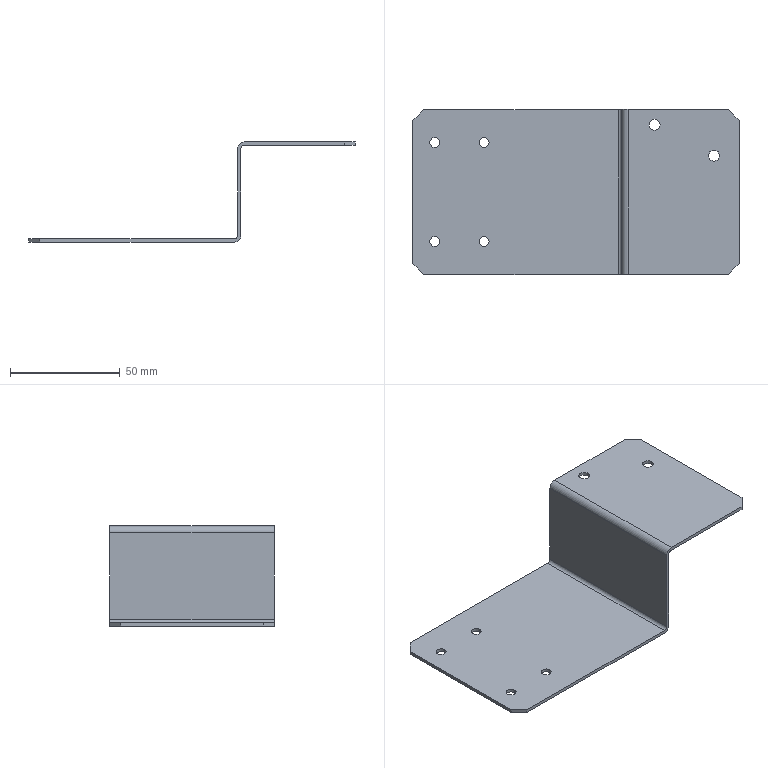Part | STEP file | 866-BDO024-96-03A_default | 1 solid | 30 faces | box 148.5 x 75 x 45.5 mm | volume 21210 mm3 | cylinder 16 | plane 14 | commonest cylinder face diameters 4.5 x8 5 x4 3 x2 6 x2
STEP:
#1=CARTESIAN_POINT('',(-66.25,15.,-42.5));
#2=VERTEX_POINT('',#1);
#3=CARTESIAN_POINT('',(-61.75,15.,-42.5));
#4=VERTEX_POINT('',#3);
#5=CARTESIAN_POINT('',(-64.,15.,-42.5));
#6=DIRECTION('',(0.,0.,1.));
#7=DIRECTION('',(-1.,0.,0.));
#8=AXIS2_PLACEMENT_3D('',#5,#6,#7);
#9=CIRCLE('',#8,2.25);
#10=EDGE_CURVE('',#2,#4,#9,.T.);
#11=ORIENTED_EDGE('',*,*,#10,.T.);
#12=CARTESIAN_POINT('',(-61.75,15.,-44.));
#13=VERTEX_POINT('',#12);
#14=CARTESIAN_POINT('',(-61.75,15.,-34.));
#15=DIRECTION('',(0.,0.,-1.));
#16=VECTOR('',#15,1000.);
#17=LINE('',#14,#16);
#18=EDGE_CURVE('',#4,#13,#17,.T.);
#19=ORIENTED_EDGE('',*,*,#18,.T.);
#20=CARTESIAN_POINT('',(-66.25,15.,-44.));
#21=VERTEX_POINT('',#20);
#22=CARTESIAN_POINT('',(-64.,15.,-44.));
#23=DIRECTION('',(0.,0.,1.));
#24=DIRECTION('',(-1.,0.,0.));
#25=AXIS2_PLACEMENT_3D('',#22,#23,#24);
#26=CIRCLE('',#25,2.25);
#27=EDGE_CURVE('',#21,#13,#26,.T.);
#28=ORIENTED_EDGE('',*,*,#27,.F.);
#29=CARTESIAN_POINT('',(-66.25,15.,-34.));
#30=DIRECTION('',(0.,0.,-1.));
#31=VECTOR('',#30,1000.);
#32=LINE('',#29,#31);
#33=EDGE_CURVE('',#2,#21,#32,.T.);
#34=ORIENTED_EDGE('',*,*,#33,.F.);
#35=EDGE_LOOP('',(#11,#19,#28,#34));
#36=FACE_OUTER_BOUND('',#35,.T.);
#37=CARTESIAN_POINT('',(-64.,15.,-34.));
#38=DIRECTION('',(0.,0.,-1.));
#39=DIRECTION('',(-1.,0.,0.));
#40=AXIS2_PLACEMENT_3D('',#37,#38,#39);
#41=CYLINDRICAL_SURFACE('',#40,2.25);
#42=ADVANCED_FACE('',(#36),#41,.F.);
#43=CARTESIAN_POINT('',(-66.25,60.,-42.5));
#44=VERTEX_POINT('',#43);
#45=CARTESIAN_POINT('',(-61.75,60.,-42.5));
#46=VERTEX_POINT('',#45);
#47=CARTESIAN_POINT('',(-64.,60.,-42.5));
#48=DIRECTION('',(0.,0.,1.));
#49=DIRECTION('',(-1.,0.,0.));
#50=AXIS2_PLACEMENT_3D('',#47,#48,#49);
#51=CIRCLE('',#50,2.25);
#52=EDGE_CURVE('',#44,#46,#51,.T.);
#53=ORIENTED_EDGE('',*,*,#52,.T.);
#54=CARTESIAN_POINT('',(-61.75,60.,-44.));
#55=VERTEX_POINT('',#54);
#56=CARTESIAN_POINT('',(-61.75,60.,-34.));
#57=DIRECTION('',(0.,0.,-1.));
#58=VECTOR('',#57,1000.);
#59=LINE('',#56,#58);
#60=EDGE_CURVE('',#46,#55,#59,.T.);
#61=ORIENTED_EDGE('',*,*,#60,.T.);
#62=CARTESIAN_POINT('',(-66.25,60.,-44.));
#63=VERTEX_POINT('',#62);
#64=CARTESIAN_POINT('',(-64.,60.,-44.));
#65=DIRECTION('',(0.,0.,1.));
#66=DIRECTION('',(-1.,0.,0.));
#67=AXIS2_PLACEMENT_3D('',#64,#65,#66);
#68=CIRCLE('',#67,2.25);
#69=EDGE_CURVE('',#63,#55,#68,.T.);
#70=ORIENTED_EDGE('',*,*,#69,.F.);
#71=CARTESIAN_POINT('',(-66.25,60.,-34.));
#72=DIRECTION('',(0.,0.,-1.));
#73=VECTOR('',#72,1000.);
#74=LINE('',#71,#73);
#75=EDGE_CURVE('',#44,#63,#74,.T.);
#76=ORIENTED_EDGE('',*,*,#75,.F.);
#77=EDGE_LOOP('',(#53,#61,#70,#76));
#78=FACE_OUTER_BOUND('',#77,.T.);
#79=CARTESIAN_POINT('',(-64.,60.,-34.));
#80=DIRECTION('',(0.,0.,-1.));
#81=DIRECTION('',(-1.,0.,0.));
#82=AXIS2_PLACEMENT_3D('',#79,#80,#81);
#83=CYLINDRICAL_SURFACE('',#82,2.25);
#84=ADVANCED_FACE('',(#78),#83,.F.);
#85=CARTESIAN_POINT('',(-88.75,15.,-42.5));
#86=VERTEX_POINT('',#85);
#87=CARTESIAN_POINT('',(-84.25,15.,-42.5));
#88=VERTEX_POINT('',#87);
#89=CARTESIAN_POINT('',(-86.5,15.,-42.5));
#90=DIRECTION('',(0.,0.,1.));
#91=DIRECTION('',(-1.,0.,0.));
#92=AXIS2_PLACEMENT_3D('',#89,#90,#91);
#93=CIRCLE('',#92,2.25);
#94=EDGE_CURVE('',#86,#88,#93,.T.);
#95=ORIENTED_EDGE('',*,*,#94,.T.);
#96=CARTESIAN_POINT('',(-84.25,15.,-44.));
#97=VERTEX_POINT('',#96);
#98=CARTESIAN_POINT('',(-84.25,15.,-34.));
#99=DIRECTION('',(0.,0.,-1.));
#100=VECTOR('',#99,1000.);
#101=LINE('',#98,#100);
#102=EDGE_CURVE('',#88,#97,#101,.T.);
#103=ORIENTED_EDGE('',*,*,#102,.T.);
#104=CARTESIAN_POINT('',(-88.75,15.,-44.));
#105=VERTEX_POINT('',#104);
#106=CARTESIAN_POINT('',(-86.5,15.,-44.));
#107=DIRECTION('',(0.,0.,1.));
#108=DIRECTION('',(-1.,0.,0.));
#109=AXIS2_PLACEMENT_3D('',#106,#107,#108);
#110=CIRCLE('',#109,2.25);
#111=EDGE_CURVE('',#105,#97,#110,.T.);
#112=ORIENTED_EDGE('',*,*,#111,.F.);
#113=CARTESIAN_POINT('',(-88.75,15.,-34.));
#114=DIRECTION('',(0.,0.,-1.));
#115=VECTOR('',#114,1000.);
#116=LINE('',#113,#115);
#117=EDGE_CURVE('',#86,#105,#116,.T.);
#118=ORIENTED_EDGE('',*,*,#117,.F.);
#119=EDGE_LOOP('',(#95,#103,#112,#118));
#120=FACE_OUTER_BOUND('',#119,.T.);
#121=CARTESIAN_POINT('',(-86.5,15.,-34.));
#122=DIRECTION('',(0.,0.,-1.));
#123=DIRECTION('',(-1.,0.,0.));
#124=AXIS2_PLACEMENT_3D('',#121,#122,#123);
#125=CYLINDRICAL_SURFACE('',#124,2.25);
#126=ADVANCED_FACE('',(#120),#125,.F.);
#127=CARTESIAN_POINT('',(-88.75,60.,-42.5));
#128=VERTEX_POINT('',#127);
#129=CARTESIAN_POINT('',(-84.25,60.,-42.5));
#130=VERTEX_POINT('',#129);
#131=CARTESIAN_POINT('',(-86.5,60.,-42.5));
#132=DIRECTION('',(0.,0.,1.));
#133=DIRECTION('',(-1.,0.,0.));
#134=AXIS2_PLACEMENT_3D('',#131,#132,#133);
#135=CIRCLE('',#134,2.25);
#136=EDGE_CURVE('',#128,#130,#135,.T.);
#137=ORIENTED_EDGE('',*,*,#136,.T.);
#138=CARTESIAN_POINT('',(-84.25,60.,-44.));
#139=VERTEX_POINT('',#138);
#140=CARTESIAN_POINT('',(-84.25,60.,-34.));
#141=DIRECTION('',(0.,0.,-1.));
#142=VECTOR('',#141,1000.);
#143=LINE('',#140,#142);
#144=EDGE_CURVE('',#130,#139,#143,.T.);
#145=ORIENTED_EDGE('',*,*,#144,.T.);
#146=CARTESIAN_POINT('',(-88.75,60.,-44.));
#147=VERTEX_POINT('',#146);
#148=CARTESIAN_POINT('',(-86.5,60.,-44.));
#149=DIRECTION('',(0.,0.,1.));
#150=DIRECTION('',(-1.,0.,0.));
#151=AXIS2_PLACEMENT_3D('',#148,#149,#150);
#152=CIRCLE('',#151,2.25);
#153=EDGE_CURVE('',#147,#139,#152,.T.);
#154=ORIENTED_EDGE('',*,*,#153,.F.);
#155=CARTESIAN_POINT('',(-88.75,60.,-34.));
#156=DIRECTION('',(0.,0.,-1.));
#157=VECTOR('',#156,1000.);
#158=LINE('',#155,#157);
#159=EDGE_CURVE('',#128,#147,#158,.T.);
#160=ORIENTED_EDGE('',*,*,#159,.F.);
#161=EDGE_LOOP('',(#137,#145,#154,#160));
#162=FACE_OUTER_BOUND('',#161,.T.);
#163=CARTESIAN_POINT('',(-86.5,60.,-34.));
#164=DIRECTION('',(0.,0.,-1.));
#165=DIRECTION('',(-1.,0.,0.));
#166=AXIS2_PLACEMENT_3D('',#163,#164,#165);
#167=CYLINDRICAL_SURFACE('',#166,2.25);
#168=ADVANCED_FACE('',(#162),#167,.F.);
#169=CARTESIAN_POINT('',(38.,54.,1.5));
#170=VERTEX_POINT('',#169);
#171=CARTESIAN_POINT('',(43.,54.,1.5));
#172=VERTEX_POINT('',#171);
#173=CARTESIAN_POINT('',(40.5,54.,1.5));
#174=DIRECTION('',(0.,0.,1.));
#175=DIRECTION('',(-1.,0.,0.));
#176=AXIS2_PLACEMENT_3D('',#173,#174,#175);
#177=CIRCLE('',#176,2.5);
#178=EDGE_CURVE('',#170,#172,#177,.T.);
#179=ORIENTED_EDGE('',*,*,#178,.T.);
#180=CARTESIAN_POINT('',(43.,54.,0.));
#181=VERTEX_POINT('',#180);
#182=CARTESIAN_POINT('',(43.,54.,0.));
#183=DIRECTION('',(0.,0.,-1.));
#184=VECTOR('',#183,1000.);
#185=LINE('',#182,#184);
#186=EDGE_CURVE('',#172,#181,#185,.T.);
#187=ORIENTED_EDGE('',*,*,#186,.T.);
#188=CARTESIAN_POINT('',(38.,54.,0.));
#189=VERTEX_POINT('',#188);
#190=CARTESIAN_POINT('',(40.5,54.,0.));
#191=DIRECTION('',(0.,0.,1.));
#192=DIRECTION('',(-1.,0.,0.));
#193=AXIS2_PLACEMENT_3D('',#190,#191,#192);
#194=CIRCLE('',#193,2.5);
#195=EDGE_CURVE('',#189,#181,#194,.T.);
#196=ORIENTED_EDGE('',*,*,#195,.F.);
#197=CARTESIAN_POINT('',(38.,54.,0.));
#198=DIRECTION('',(0.,0.,-1.));
#199=VECTOR('',#198,1000.);
#200=LINE('',#197,#199);
#201=EDGE_CURVE('',#170,#189,#200,.T.);
#202=ORIENTED_EDGE('',*,*,#201,.F.);
#203=EDGE_LOOP('',(#179,#187,#196,#202));
#204=FACE_OUTER_BOUND('',#203,.T.);
#205=CARTESIAN_POINT('',(40.5,54.,0.));
#206=DIRECTION('',(0.,0.,-1.));
#207=DIRECTION('',(-1.,0.,0.));
#208=AXIS2_PLACEMENT_3D('',#205,#206,#207);
#209=CYLINDRICAL_SURFACE('',#208,2.5);
#210=ADVANCED_FACE('',(#204),#209,.F.);
#211=CARTESIAN_POINT('',(11.,68.,1.5));
#212=VERTEX_POINT('',#211);
#213=CARTESIAN_POINT('',(16.,68.,1.5));
#214=VERTEX_POINT('',#213);
#215=CARTESIAN_POINT('',(13.5,68.,1.5));
#216=DIRECTION('',(0.,0.,1.));
#217=DIRECTION('',(-1.,0.,0.));
#218=AXIS2_PLACEMENT_3D('',#215,#216,#217);
#219=CIRCLE('',#218,2.5);
#220=EDGE_CURVE('',#212,#214,#219,.T.);
#221=ORIENTED_EDGE('',*,*,#220,.T.);
#222=CARTESIAN_POINT('',(16.,68.,0.));
#223=VERTEX_POINT('',#222);
#224=CARTESIAN_POINT('',(16.,68.,0.));
#225=DIRECTION('',(0.,0.,-1.));
#226=VECTOR('',#225,1000.);
#227=LINE('',#224,#226);
#228=EDGE_CURVE('',#214,#223,#227,.T.);
#229=ORIENTED_EDGE('',*,*,#228,.T.);
#230=CARTESIAN_POINT('',(11.,68.,0.));
#231=VERTEX_POINT('',#230);
#232=CARTESIAN_POINT('',(13.5,68.,0.));
#233=DIRECTION('',(0.,0.,1.));
#234=DIRECTION('',(-1.,0.,0.));
#235=AXIS2_PLACEMENT_3D('',#232,#233,#234);
#236=CIRCLE('',#235,2.5);
#237=EDGE_CURVE('',#231,#223,#236,.T.);
#238=ORIENTED_EDGE('',*,*,#237,.F.);
#239=CARTESIAN_POINT('',(11.,68.,0.));
#240=DIRECTION('',(0.,0.,-1.));
#241=VECTOR('',#240,1000.);
#242=LINE('',#239,#241);
#243=EDGE_CURVE('',#212,#231,#242,.T.);
#244=ORIENTED_EDGE('',*,*,#243,.F.);
#245=EDGE_LOOP('',(#221,#229,#238,#244));
#246=FACE_OUTER_BOUND('',#245,.T.);
#247=CARTESIAN_POINT('',(13.5,68.,0.));
#248=DIRECTION('',(0.,0.,-1.));
#249=DIRECTION('',(-1.,0.,0.));
#250=AXIS2_PLACEMENT_3D('',#247,#248,#249);
#251=CYLINDRICAL_SURFACE('',#250,2.5);
#252=ADVANCED_FACE('',(#246),#251,.F.);
#253=CARTESIAN_POINT('',(-91.5,0.,-42.5));
#254=VERTEX_POINT('',#253);
#255=CARTESIAN_POINT('',(-96.5,5.,-42.5));
#256=VERTEX_POINT('',#255);
#257=CARTESIAN_POINT('',(-91.5,0.,-42.5));
#258=DIRECTION('',(-0.7071,0.7071,0.));
#259=VECTOR('',#258,1000.);
#260=LINE('',#257,#259);
#261=EDGE_CURVE('',#254,#256,#260,.T.);
#262=ORIENTED_EDGE('',*,*,#261,.F.);
#263=CARTESIAN_POINT('',(-3.,0.,-42.5));
#264=VERTEX_POINT('',#263);
#265=CARTESIAN_POINT('',(-96.5,0.,-42.5));
#266=DIRECTION('',(-1.,0.,0.));
#267=VECTOR('',#266,1000.);
#268=LINE('',#265,#267);
#269=EDGE_CURVE('',#264,#254,#268,.T.);
#270=ORIENTED_EDGE('',*,*,#269,.F.);
#271=CARTESIAN_POINT('',(-3.,75.,-42.5));
#272=VERTEX_POINT('',#271);
#273=CARTESIAN_POINT('',(-3.,75.,-42.5));
#274=DIRECTION('',(0.,-1.,0.));
#275=VECTOR('',#274,1000.);
#276=LINE('',#273,#275);
#277=EDGE_CURVE('',#272,#264,#276,.T.);
#278=ORIENTED_EDGE('',*,*,#277,.F.);
#279=CARTESIAN_POINT('',(-91.5,75.,-42.5));
#280=VERTEX_POINT('',#279);
#281=CARTESIAN_POINT('',(-96.5,75.,-42.5));
#282=DIRECTION('',(1.,0.,0.));
#283=VECTOR('',#282,1000.);
#284=LINE('',#281,#283);
#285=EDGE_CURVE('',#280,#272,#284,.T.);
#286=ORIENTED_EDGE('',*,*,#285,.F.);
#287=CARTESIAN_POINT('',(-96.5,70.,-42.5));
#288=VERTEX_POINT('',#287);
#289=CARTESIAN_POINT('',(-96.5,70.,-42.5));
#290=DIRECTION('',(0.7071,0.7071,0.));
#291=VECTOR('',#290,1000.);
#292=LINE('',#289,#291);
#293=EDGE_CURVE('',#288,#280,#292,.T.);
#294=ORIENTED_EDGE('',*,*,#293,.F.);
#295=CARTESIAN_POINT('',(-96.5,75.,-42.5));
#296=DIRECTION('',(0.,1.,0.));
#297=VECTOR('',#296,1000.);
#298=LINE('',#295,#297);
#299=EDGE_CURVE('',#256,#288,#298,.T.);
#300=ORIENTED_EDGE('',*,*,#299,.F.);
#301=EDGE_LOOP('',(#262,#270,#278,#286,#294,#300));
#302=FACE_OUTER_BOUND('',#301,.T.);
#303=ORIENTED_EDGE('',*,*,#10,.F.);
#304=CARTESIAN_POINT('',(-64.,15.,-42.5));
#305=DIRECTION('',(0.,0.,1.));
#306=DIRECTION('',(-1.,0.,0.));
#307=AXIS2_PLACEMENT_3D('',#304,#305,#306);
#308=CIRCLE('',#307,2.25);
#309=EDGE_CURVE('',#4,#2,#308,.T.);
#310=ORIENTED_EDGE('',*,*,#309,.F.);
#311=EDGE_LOOP('',(#303,#310));
#312=FACE_BOUND('',#311,.T.);
#313=ORIENTED_EDGE('',*,*,#52,.F.);
#314=CARTESIAN_POINT('',(-64.,60.,-42.5));
#315=DIRECTION('',(0.,0.,1.));
#316=DIRECTION('',(-1.,0.,0.));
#317=AXIS2_PLACEMENT_3D('',#314,#315,#316);
#318=CIRCLE('',#317,2.25);
#319=EDGE_CURVE('',#46,#44,#318,.T.);
#320=ORIENTED_EDGE('',*,*,#319,.F.);
#321=EDGE_LOOP('',(#313,#320));
#322=FACE_BOUND('',#321,.T.);
#323=ORIENTED_EDGE('',*,*,#94,.F.);
#324=CARTESIAN_POINT('',(-86.5,15.,-42.5));
#325=DIRECTION('',(0.,0.,1.));
#326=DIRECTION('',(-1.,0.,0.));
#327=AXIS2_PLACEMENT_3D('',#324,#325,#326);
#328=CIRCLE('',#327,2.25);
#329=EDGE_CURVE('',#88,#86,#328,.T.);
#330=ORIENTED_EDGE('',*,*,#329,.F.);
#331=EDGE_LOOP('',(#323,#330));
#332=FACE_BOUND('',#331,.T.);
#333=ORIENTED_EDGE('',*,*,#136,.F.);
#334=CARTESIAN_POINT('',(-86.5,60.,-42.5));
#335=DIRECTION('',(0.,0.,1.));
#336=DIRECTION('',(-1.,0.,0.));
#337=AXIS2_PLACEMENT_3D('',#334,#335,#336);
#338=CIRCLE('',#337,2.25);
#339=EDGE_CURVE('',#130,#128,#338,.T.);
#340=ORIENTED_EDGE('',*,*,#339,.F.);
#341=EDGE_LOOP('',(#333,#340));
#342=FACE_BOUND('',#341,.T.);
#343=CARTESIAN_POINT('',(-96.5,75.,-42.5));
#344=DIRECTION('',(0.,0.,-1.));
#345=DIRECTION('',(-1.,0.,0.));
#346=AXIS2_PLACEMENT_3D('',#343,#344,#345);
#347=PLANE('',#346);
#348=ADVANCED_FACE('',(#302,#312,#322,#332,#342),#347,.F.);
#349=ORIENTED_EDGE('',*,*,#299,.T.);
#350=CARTESIAN_POINT('',(-96.5,70.,-44.));
#351=VERTEX_POINT('',#350);
#352=CARTESIAN_POINT('',(-96.5,70.,-42.5));
#353=DIRECTION('',(0.,0.,-1.));
#354=VECTOR('',#353,1000.);
#355=LINE('',#352,#354);
#356=EDGE_CURVE('',#288,#351,#355,.T.);
#357=ORIENTED_EDGE('',*,*,#356,.T.);
#358=CARTESIAN_POINT('',(-96.5,5.,-44.));
#359=VERTEX_POINT('',#358);
#360=CARTESIAN_POINT('',(-96.5,75.,-44.));
#361=DIRECTION('',(0.,-1.,0.));
#362=VECTOR('',#361,1000.);
#363=LINE('',#360,#362);
#364=EDGE_CURVE('',#351,#359,#363,.T.);
#365=ORIENTED_EDGE('',*,*,#364,.T.);
#366=CARTESIAN_POINT('',(-96.5,5.,-42.5));
#367=DIRECTION('',(0.,0.,1.));
#368=VECTOR('',#367,1000.);
#369=LINE('',#366,#368);
#370=EDGE_CURVE('',#359,#256,#369,.T.);
#371=ORIENTED_EDGE('',*,*,#370,.T.);
#372=EDGE_LOOP('',(#349,#357,#365,#371));
#373=FACE_OUTER_BOUND('',#372,.T.);
#374=CARTESIAN_POINT('',(-96.5,75.,-42.5));
#375=DIRECTION('',(-1.,0.,0.));
#376=DIRECTION('',(0.,0.,1.));
#377=AXIS2_PLACEMENT_3D('',#374,#375,#376);
#378=PLANE('',#377);
#379=ADVANCED_FACE('',(#373),#378,.T.);
#380=ORIENTED_EDGE('',*,*,#370,.F.);
#381=CARTESIAN_POINT('',(-91.5,0.,-44.));
#382=VERTEX_POINT('',#381);
#383=CARTESIAN_POINT('',(-91.5,0.,-44.));
#384=DIRECTION('',(-0.7071,0.7071,0.));
#385=VECTOR('',#384,1000.);
#386=LINE('',#383,#385);
#387=EDGE_CURVE('',#382,#359,#386,.T.);
#388=ORIENTED_EDGE('',*,*,#387,.F.);
#389=CARTESIAN_POINT('',(-91.5,0.,-41.));
#390=DIRECTION('',(0.,0.,-1.));
#391=VECTOR('',#390,1000.);
#392=LINE('',#389,#391);
#393=EDGE_CURVE('',#254,#382,#392,.T.);
#394=ORIENTED_EDGE('',*,*,#393,.F.);
#395=ORIENTED_EDGE('',*,*,#261,.T.);
#396=EDGE_LOOP('',(#380,#388,#394,#395));
#397=FACE_OUTER_BOUND('',#396,.T.);
#398=CARTESIAN_POINT('',(-91.5,0.,-41.));
#399=DIRECTION('',(0.7071,0.7071,0.));
#400=DIRECTION('',(-0.7071,0.7071,0.));
#401=AXIS2_PLACEMENT_3D('',#398,#399,#400);
#402=PLANE('',#401);
#403=ADVANCED_FACE('',(#397),#402,.F.);
#404=CARTESIAN_POINT('',(-3.,0.,-44.));
#405=VERTEX_POINT('',#404);
#406=CARTESIAN_POINT('',(-1.5,0.,-44.));
#407=DIRECTION('',(1.,0.,0.));
#408=VECTOR('',#407,1000.);
#409=LINE('',#406,#408);
#410=EDGE_CURVE('',#382,#405,#409,.T.);
#411=ORIENTED_EDGE('',*,*,#410,.T.);
#412=CARTESIAN_POINT('',(0.,0.,-41.));
#413=VERTEX_POINT('',#412);
#414=CARTESIAN_POINT('',(-3.,0.,-41.));
#415=DIRECTION('',(0.,-1.,0.));
#416=DIRECTION('',(0.,0.,-1.));
#417=AXIS2_PLACEMENT_3D('',#414,#415,#416);
#418=CIRCLE('',#417,3.);
#419=EDGE_CURVE('',#405,#413,#418,.T.);
#420=ORIENTED_EDGE('',*,*,#419,.T.);
#421=CARTESIAN_POINT('',(0.,0.,-1.5));
#422=VERTEX_POINT('',#421);
#423=CARTESIAN_POINT('',(0.,0.,1.5));
#424=DIRECTION('',(0.,0.,1.));
#425=VECTOR('',#424,1000.);
#426=LINE('',#423,#425);
#427=EDGE_CURVE('',#413,#422,#426,.T.);
#428=ORIENTED_EDGE('',*,*,#427,.T.);
#429=CARTESIAN_POINT('',(1.5,0.,0.));
#430=VERTEX_POINT('',#429);
#431=CARTESIAN_POINT('',(1.5,0.,-1.5));
#432=DIRECTION('',(0.,1.,0.));
#433=DIRECTION('',(0.,0.,-1.));
#434=AXIS2_PLACEMENT_3D('',#431,#432,#433);
#435=CIRCLE('',#434,1.5);
#436=EDGE_CURVE('',#422,#430,#435,.T.);
#437=ORIENTED_EDGE('',*,*,#436,.T.);
#438=CARTESIAN_POINT('',(47.,0.,0.));
#439=VERTEX_POINT('',#438);
#440=CARTESIAN_POINT('',(1.5,0.,0.));
#441=DIRECTION('',(1.,0.,0.));
#442=VECTOR('',#441,1000.);
#443=LINE('',#440,#442);
#444=EDGE_CURVE('',#430,#439,#443,.T.);
#445=ORIENTED_EDGE('',*,*,#444,.T.);
#446=CARTESIAN_POINT('',(47.,0.,1.5));
#447=VERTEX_POINT('',#446);
#448=CARTESIAN_POINT('',(47.,0.,-1.5));
#449=DIRECTION('',(0.,0.,1.));
#450=VECTOR('',#449,1000.);
#451=LINE('',#448,#450);
#452=EDGE_CURVE('',#439,#447,#451,.T.);
#453=ORIENTED_EDGE('',*,*,#452,.T.);
#454=CARTESIAN_POINT('',(1.5,0.,1.5));
#455=VERTEX_POINT('',#454);
#456=CARTESIAN_POINT('',(0.,0.,1.5));
#457=DIRECTION('',(-1.,0.,0.));
#458=VECTOR('',#457,1000.);
#459=LINE('',#456,#458);
#460=EDGE_CURVE('',#447,#455,#459,.T.);
#461=ORIENTED_EDGE('',*,*,#460,.T.);
#462=CARTESIAN_POINT('',(-1.5,0.,-1.5));
#463=VERTEX_POINT('',#462);
#464=CARTESIAN_POINT('',(1.5,0.,-1.5));
#465=DIRECTION('',(0.,1.,0.));
#466=DIRECTION('',(0.,0.,-1.));
#467=AXIS2_PLACEMENT_3D('',#464,#465,#466);
#468=CIRCLE('',#467,3.);
#469=EDGE_CURVE('',#463,#455,#468,.T.);
#470=ORIENTED_EDGE('',*,*,#469,.F.);
#471=CARTESIAN_POINT('',(-1.5,0.,-41.));
#472=VERTEX_POINT('',#471);
#473=CARTESIAN_POINT('',(-1.5,0.,-44.));
#474=DIRECTION('',(0.,0.,-1.));
#475=VECTOR('',#474,1000.);
#476=LINE('',#473,#475);
#477=EDGE_CURVE('',#463,#472,#476,.T.);
#478=ORIENTED_EDGE('',*,*,#477,.T.);
#479=CARTESIAN_POINT('',(-3.,0.,-41.));
#480=DIRECTION('',(0.,1.,0.));
#481=DIRECTION('',(0.,0.,-1.));
#482=AXIS2_PLACEMENT_3D('',#479,#480,#481);
#483=CIRCLE('',#482,1.5);
#484=EDGE_CURVE('',#472,#264,#483,.T.);
#485=ORIENTED_EDGE('',*,*,#484,.T.);
#486=ORIENTED_EDGE('',*,*,#269,.T.);
#487=ORIENTED_EDGE('',*,*,#393,.T.);
#488=EDGE_LOOP('',(#411,#420,#428,#437,#445,#453,#461,#470,#478,#485,#486,#487));
#489=FACE_OUTER_BOUND('',#488,.T.);
#490=CARTESIAN_POINT('',(-1.5,0.,-41.));
#491=DIRECTION('',(0.,-1.,0.));
#492=DIRECTION('',(0.,0.,-1.));
#493=AXIS2_PLACEMENT_3D('',#490,#491,#492);
#494=PLANE('',#493);
#495=ADVANCED_FACE('',(#489),#494,.T.);
#496=CARTESIAN_POINT('',(-1.5,75.,-41.));
#497=VERTEX_POINT('',#496);
#498=CARTESIAN_POINT('',(-1.5,75.,-41.));
#499=DIRECTION('',(0.,-1.,0.));
#500=VECTOR('',#499,1000.);
#501=LINE('',#498,#500);
#502=EDGE_CURVE('',#497,#472,#501,.T.);
#503=ORIENTED_EDGE('',*,*,#502,.F.);
#504=CARTESIAN_POINT('',(-3.,75.,-41.));
#505=DIRECTION('',(0.,-1.,0.));
#506=DIRECTION('',(0.,0.,-1.));
#507=AXIS2_PLACEMENT_3D('',#504,#505,#506);
#508=CIRCLE('',#507,1.5);
#509=EDGE_CURVE('',#272,#497,#508,.T.);
#510=ORIENTED_EDGE('',*,*,#509,.F.);
#511=ORIENTED_EDGE('',*,*,#277,.T.);
#512=ORIENTED_EDGE('',*,*,#484,.F.);
#513=EDGE_LOOP('',(#503,#510,#511,#512));
#514=FACE_OUTER_BOUND('',#513,.T.);
#515=CARTESIAN_POINT('',(-3.,75.,-41.));
#516=DIRECTION('',(0.,-1.,0.));
#517=DIRECTION('',(0.,0.,-1.));
#518=AXIS2_PLACEMENT_3D('',#515,#516,#517);
#519=CYLINDRICAL_SURFACE('',#518,1.5);
#520=ADVANCED_FACE('',(#514),#519,.F.);
#521=CARTESIAN_POINT('',(-91.5,75.,-44.));
#522=VERTEX_POINT('',#521);
#523=CARTESIAN_POINT('',(-91.5,75.,-1.5));
#524=DIRECTION('',(0.,0.,-1.));
#525=VECTOR('',#524,1000.);
#526=LINE('',#523,#525);
#527=EDGE_CURVE('',#280,#522,#526,.T.);
#528=ORIENTED_EDGE('',*,*,#527,.F.);
#529=ORIENTED_EDGE('',*,*,#285,.T.);
#530=ORIENTED_EDGE('',*,*,#509,.T.);
#531=CARTESIAN_POINT('',(-1.5,75.,-1.5));
#532=VERTEX_POINT('',#531);
#533=CARTESIAN_POINT('',(-1.5,75.,-44.));
#534=DIRECTION('',(0.,0.,1.));
#535=VECTOR('',#534,1000.);
#536=LINE('',#533,#535);
#537=EDGE_CURVE('',#497,#532,#536,.T.);
#538=ORIENTED_EDGE('',*,*,#537,.T.);
#539=CARTESIAN_POINT('',(1.5,75.,1.5));
#540=VERTEX_POINT('',#539);
#541=CARTESIAN_POINT('',(1.5,75.,-1.5));
#542=DIRECTION('',(0.,-1.,0.));
#543=DIRECTION('',(0.,0.,-1.));
#544=AXIS2_PLACEMENT_3D('',#541,#542,#543);
#545=CIRCLE('',#544,3.);
#546=EDGE_CURVE('',#540,#532,#545,.T.);
#547=ORIENTED_EDGE('',*,*,#546,.F.);
#548=CARTESIAN_POINT('',(47.,75.,1.5));
#549=VERTEX_POINT('',#548);
#550=CARTESIAN_POINT('',(0.,75.,1.5));
#551=DIRECTION('',(1.,0.,0.));
#552=VECTOR('',#551,1000.);
#553=LINE('',#550,#552);
#554=EDGE_CURVE('',#540,#549,#553,.T.);
#555=ORIENTED_EDGE('',*,*,#554,.T.);
#556=CARTESIAN_POINT('',(47.,75.,0.));
#557=VERTEX_POINT('',#556);
#558=CARTESIAN_POINT('',(47.,75.,0.));
#559=DIRECTION('',(0.,0.,-1.));
#560=VECTOR('',#559,1000.);
#561=LINE('',#558,#560);
#562=EDGE_CURVE('',#549,#557,#561,.T.);
#563=ORIENTED_EDGE('',*,*,#562,.T.);
#564=CARTESIAN_POINT('',(1.5,75.,0.));
#565=VERTEX_POINT('',#564);
#566=CARTESIAN_POINT('',(-1.5,75.,0.));
#567=DIRECTION('',(-1.,0.,0.));
#568=VECTOR('',#567,1000.);
#569=LINE('',#566,#568);
#570=EDGE_CURVE('',#557,#565,#569,.T.);
#571=ORIENTED_EDGE('',*,*,#570,.T.);
#572=CARTESIAN_POINT('',(0.,75.,-1.5));
#573=VERTEX_POINT('',#572);
#574=CARTESIAN_POINT('',(1.5,75.,-1.5));
#575=DIRECTION('',(0.,-1.,0.));
#576=DIRECTION('',(0.,0.,-1.));
#577=AXIS2_PLACEMENT_3D('',#574,#575,#576);
#578=CIRCLE('',#577,1.5);
#579=EDGE_CURVE('',#565,#573,#578,.T.);
#580=ORIENTED_EDGE('',*,*,#579,.T.);
#581=CARTESIAN_POINT('',(0.,75.,-41.));
#582=VERTEX_POINT('',#581);
#583=CARTESIAN_POINT('',(0.,75.,-42.5));
#584=DIRECTION('',(0.,0.,-1.));
#585=VECTOR('',#584,1000.);
#586=LINE('',#583,#585);
#587=EDGE_CURVE('',#573,#582,#586,.T.);
#588=ORIENTED_EDGE('',*,*,#587,.T.);
#589=CARTESIAN_POINT('',(-3.,75.,-44.));
#590=VERTEX_POINT('',#589);
#591=CARTESIAN_POINT('',(-3.,75.,-41.));
#592=DIRECTION('',(0.,1.,0.));
#593=DIRECTION('',(0.,0.,-1.));
#594=AXIS2_PLACEMENT_3D('',#591,#592,#593);
#595=CIRCLE('',#594,3.);
#596=EDGE_CURVE('',#582,#590,#595,.T.);
#597=ORIENTED_EDGE('',*,*,#596,.T.);
#598=CARTESIAN_POINT('',(1.5,75.,-44.));
#599=DIRECTION('',(1.,0.,0.));
#600=VECTOR('',#599,1000.);
#601=LINE('',#598,#600);
#602=EDGE_CURVE('',#522,#590,#601,.T.);
#603=ORIENTED_EDGE('',*,*,#602,.F.);
#604=EDGE_LOOP('',(#528,#529,#530,#538,#547,#555,#563,#571,#580,#588,#597,#603));
#605=FACE_OUTER_BOUND('',#604,.T.);
#606=CARTESIAN_POINT('',(1.5,75.,-1.5));
#607=DIRECTION('',(0.,-1.,0.));
#608=DIRECTION('',(0.,0.,-1.));
#609=AXIS2_PLACEMENT_3D('',#606,#607,#608);
#610=PLANE('',#609);
#611=ADVANCED_FACE('',(#605),#610,.F.);
#612=CARTESIAN_POINT('',(-96.5,70.,-44.));
#613=DIRECTION('',(-0.7071,-0.7071,0.));
#614=VECTOR('',#613,1000.);
#615=LINE('',#612,#614);
#616=EDGE_CURVE('',#522,#351,#615,.T.);
#617=ORIENTED_EDGE('',*,*,#616,.T.);
#618=ORIENTED_EDGE('',*,*,#356,.F.);
#619=ORIENTED_EDGE('',*,*,#293,.T.);
#620=ORIENTED_EDGE('',*,*,#527,.T.);
#621=EDGE_LOOP('',(#617,#618,#619,#620));
#622=FACE_OUTER_BOUND('',#621,.T.);
#623=CARTESIAN_POINT('',(-96.5,70.,-42.5));
#624=DIRECTION('',(-0.7071,0.7071,0.));
#625=DIRECTION('',(-0.7071,-0.7071,0.));
#626=AXIS2_PLACEMENT_3D('',#623,#624,#625);
#627=PLANE('',#626);
#628=ADVANCED_FACE('',(#622),#627,.T.);
#629=ORIENTED_EDGE('',*,*,#18,.F.);
#630=ORIENTED_EDGE('',*,*,#309,.T.);
#631=ORIENTED_EDGE('',*,*,#33,.T.);
#632=CARTESIAN_POINT('',(-64.,15.,-44.));
#633=DIRECTION('',(0.,0.,1.));
#634=DIRECTION('',(-1.,0.,0.));
#635=AXIS2_PLACEMENT_3D('',#632,#633,#634);
#636=CIRCLE('',#635,2.25);
#637=EDGE_CURVE('',#13,#21,#636,.T.);
#638=ORIENTED_EDGE('',*,*,#637,.F.);
#639=EDGE_LOOP('',(#629,#630,#631,#638));
#640=FACE_OUTER_BOUND('',#639,.T.);
#641=CARTESIAN_POINT('',(-64.,15.,-34.));
#642=DIRECTION('',(0.,0.,-1.));
#643=DIRECTION('',(-1.,0.,0.));
#644=AXIS2_PLACEMENT_3D('',#641,#642,#643);
#645=CYLINDRICAL_SURFACE('',#644,2.25);
#646=ADVANCED_FACE('',(#640),#645,.F.);
#647=ORIENTED_EDGE('',*,*,#60,.F.);
#648=ORIENTED_EDGE('',*,*,#319,.T.);
#649=ORIENTED_EDGE('',*,*,#75,.T.);
#650=CARTESIAN_POINT('',(-64.,60.,-44.));
#651=DIRECTION('',(0.,0.,1.));
#652=DIRECTION('',(-1.,0.,0.));
#653=AXIS2_PLACEMENT_3D('',#650,#651,#652);
#654=CIRCLE('',#653,2.25);
#655=EDGE_CURVE('',#55,#63,#654,.T.);
#656=ORIENTED_EDGE('',*,*,#655,.F.);
#657=EDGE_LOOP('',(#647,#648,#649,#656));
#658=FACE_OUTER_BOUND('',#657,.T.);
#659=CARTESIAN_POINT('',(-64.,60.,-34.));
#660=DIRECTION('',(0.,0.,-1.));
#661=DIRECTION('',(-1.,0.,0.));
#662=AXIS2_PLACEMENT_3D('',#659,#660,#661);
#663=CYLINDRICAL_SURFACE('',#662,2.25);
#664=ADVANCED_FACE('',(#658),#663,.F.);
#665=ORIENTED_EDGE('',*,*,#102,.F.);
#666=ORIENTED_EDGE('',*,*,#329,.T.);
#667=ORIENTED_EDGE('',*,*,#117,.T.);
#668=CARTESIAN_POINT('',(-86.5,15.,-44.));
#669=DIRECTION('',(0.,0.,1.));
#670=DIRECTION('',(-1.,0.,0.));
#671=AXIS2_PLACEMENT_3D('',#668,#669,#670);
#672=CIRCLE('',#671,2.25);
#673=EDGE_CURVE('',#97,#105,#672,.T.);
#674=ORIENTED_EDGE('',*,*,#673,.F.);
#675=EDGE_LOOP('',(#665,#666,#667,#674));
#676=FACE_OUTER_BOUND('',#675,.T.);
#677=CARTESIAN_POINT('',(-86.5,15.,-34.));
#678=DIRECTION('',(0.,0.,-1.));
#679=DIRECTION('',(-1.,0.,0.));
#680=AXIS2_PLACEMENT_3D('',#677,#678,#679);
#681=CYLINDRICAL_SURFACE('',#680,2.25);
#682=ADVANCED_FACE('',(#676),#681,.F.);
#683=ORIENTED_EDGE('',*,*,#144,.F.);
#684=ORIENTED_EDGE('',*,*,#339,.T.);
#685=ORIENTED_EDGE('',*,*,#159,.T.);
#686=CARTESIAN_POINT('',(-86.5,60.,-44.));
#687=DIRECTION('',(0.,0.,1.));
#688=DIRECTION('',(-1.,0.,0.));
#689=AXIS2_PLACEMENT_3D('',#686,#687,#688);
#690=CIRCLE('',#689,2.25);
#691=EDGE_CURVE('',#139,#147,#690,.T.);
#692=ORIENTED_EDGE('',*,*,#691,.F.);
#693=EDGE_LOOP('',(#683,#684,#685,#692));
#694=FACE_OUTER_BOUND('',#693,.T.);
#695=CARTESIAN_POINT('',(-86.5,60.,-34.));
#696=DIRECTION('',(0.,0.,-1.));
#697=DIRECTION('',(-1.,0.,0.));
#698=AXIS2_PLACEMENT_3D('',#695,#696,#697);
#699=CYLINDRICAL_SURFACE('',#698,2.25);
#700=ADVANCED_FACE('',(#694),#699,.F.);
#701=ORIENTED_EDGE('',*,*,#602,.T.);
#702=CARTESIAN_POINT('',(-3.,75.,-44.));
#703=DIRECTION('',(0.,-1.,0.));
#704=VECTOR('',#703,1000.);
#705=LINE('',#702,#704);
#706=EDGE_CURVE('',#590,#405,#705,.T.);
#707=ORIENTED_EDGE('',*,*,#706,.T.);
#708=ORIENTED_EDGE('',*,*,#410,.F.);
#709=ORIENTED_EDGE('',*,*,#387,.T.);
#710=ORIENTED_EDGE('',*,*,#364,.F.);
#711=ORIENTED_EDGE('',*,*,#616,.F.);
#712=EDGE_LOOP('',(#701,#707,#708,#709,#710,#711));
#713=FACE_OUTER_BOUND('',#712,.T.);
#714=ORIENTED_EDGE('',*,*,#27,.T.);
#715=ORIENTED_EDGE('',*,*,#637,.T.);
#716=EDGE_LOOP('',(#714,#715));
#717=FACE_BOUND('',#716,.T.);
#718=ORIENTED_EDGE('',*,*,#69,.T.);
#719=ORIENTED_EDGE('',*,*,#655,.T.);
#720=EDGE_LOOP('',(#718,#719));
#721=FACE_BOUND('',#720,.T.);
#722=ORIENTED_EDGE('',*,*,#111,.T.);
#723=ORIENTED_EDGE('',*,*,#673,.T.);
#724=EDGE_LOOP('',(#722,#723));
#725=FACE_BOUND('',#724,.T.);
#726=ORIENTED_EDGE('',*,*,#153,.T.);
#727=ORIENTED_EDGE('',*,*,#691,.T.);
#728=EDGE_LOOP('',(#726,#727));
#729=FACE_BOUND('',#728,.T.);
#730=CARTESIAN_POINT('',(-96.5,75.,-44.));
#731=DIRECTION('',(0.,0.,-1.));
#732=DIRECTION('',(-1.,0.,0.));
#733=AXIS2_PLACEMENT_3D('',#730,#731,#732);
#734=PLANE('',#733);
#735=ADVANCED_FACE('',(#713,#717,#721,#725,#729),#734,.T.);
#736=CARTESIAN_POINT('',(-1.5,75.,-1.5));
#737=DIRECTION('',(0.,-1.,0.));
#738=VECTOR('',#737,1000.);
#739=LINE('',#736,#738);
#740=EDGE_CURVE('',#532,#463,#739,.T.);
#741=ORIENTED_EDGE('',*,*,#740,.F.);
#742=ORIENTED_EDGE('',*,*,#537,.F.);
#743=ORIENTED_EDGE('',*,*,#502,.T.);
#744=ORIENTED_EDGE('',*,*,#477,.F.);
#745=EDGE_LOOP('',(#741,#742,#743,#744));
#746=FACE_OUTER_BOUND('',#745,.T.);
#747=CARTESIAN_POINT('',(-1.5,75.,-44.));
#748=DIRECTION('',(1.,0.,0.));
#749=DIRECTION('',(0.,0.,-1.));
#750=AXIS2_PLACEMENT_3D('',#747,#748,#749);
#751=PLANE('',#750);
#752=ADVANCED_FACE('',(#746),#751,.F.);
#753=ORIENTED_EDGE('',*,*,#596,.F.);
#754=CARTESIAN_POINT('',(0.,75.,-41.));
#755=DIRECTION('',(0.,-1.,0.));
#756=VECTOR('',#755,1000.);
#757=LINE('',#754,#756);
#758=EDGE_CURVE('',#582,#413,#757,.T.);
#759=ORIENTED_EDGE('',*,*,#758,.T.);
#760=ORIENTED_EDGE('',*,*,#419,.F.);
#761=ORIENTED_EDGE('',*,*,#706,.F.);
#762=EDGE_LOOP('',(#753,#759,#760,#761));
#763=FACE_OUTER_BOUND('',#762,.T.);
#764=CARTESIAN_POINT('',(-3.,75.,-41.));
#765=DIRECTION('',(0.,-1.,0.));
#766=DIRECTION('',(0.,0.,-1.));
#767=AXIS2_PLACEMENT_3D('',#764,#765,#766);
#768=CYLINDRICAL_SURFACE('',#767,3.);
#769=ADVANCED_FACE('',(#763),#768,.T.);
#770=ORIENTED_EDGE('',*,*,#546,.T.);
#771=ORIENTED_EDGE('',*,*,#740,.T.);
#772=ORIENTED_EDGE('',*,*,#469,.T.);
#773=CARTESIAN_POINT('',(1.5,75.,1.5));
#774=DIRECTION('',(0.,1.,0.));
#775=VECTOR('',#774,1000.);
#776=LINE('',#773,#775);
#777=EDGE_CURVE('',#455,#540,#776,.T.);
#778=ORIENTED_EDGE('',*,*,#777,.T.);
#779=EDGE_LOOP('',(#770,#771,#772,#778));
#780=FACE_OUTER_BOUND('',#779,.T.);
#781=CARTESIAN_POINT('',(1.5,75.,-1.5));
#782=DIRECTION('',(0.,-1.,0.));
#783=DIRECTION('',(0.,0.,-1.));
#784=AXIS2_PLACEMENT_3D('',#781,#782,#783);
#785=CYLINDRICAL_SURFACE('',#784,3.);
#786=ADVANCED_FACE('',(#780),#785,.T.);
#787=ORIENTED_EDGE('',*,*,#587,.F.);
#788=CARTESIAN_POINT('',(0.,75.,-1.5));
#789=DIRECTION('',(0.,-1.,0.));
#790=VECTOR('',#789,1000.);
#791=LINE('',#788,#790);
#792=EDGE_CURVE('',#573,#422,#791,.T.);
#793=ORIENTED_EDGE('',*,*,#792,.T.);
#794=ORIENTED_EDGE('',*,*,#427,.F.);
#795=ORIENTED_EDGE('',*,*,#758,.F.);
#796=EDGE_LOOP('',(#787,#793,#794,#795));
#797=FACE_OUTER_BOUND('',#796,.T.);
#798=CARTESIAN_POINT('',(0.,75.,-44.));
#799=DIRECTION('',(1.,0.,0.));
#800=DIRECTION('',(0.,0.,-1.));
#801=AXIS2_PLACEMENT_3D('',#798,#799,#800);
#802=PLANE('',#801);
#803=ADVANCED_FACE('',(#797),#802,.T.);
#804=CARTESIAN_POINT('',(52.,70.,1.5));
#805=VERTEX_POINT('',#804);
#806=CARTESIAN_POINT('',(47.,75.,1.5));
#807=DIRECTION('',(0.7071,-0.7071,0.));
#808=VECTOR('',#807,1000.);
#809=LINE('',#806,#808);
#810=EDGE_CURVE('',#549,#805,#809,.T.);
#811=ORIENTED_EDGE('',*,*,#810,.F.);
#812=ORIENTED_EDGE('',*,*,#554,.F.);
#813=ORIENTED_EDGE('',*,*,#777,.F.);
#814=ORIENTED_EDGE('',*,*,#460,.F.);
#815=CARTESIAN_POINT('',(52.,5.,1.5));
#816=VERTEX_POINT('',#815);
#817=CARTESIAN_POINT('',(52.,5.,1.5));
#818=DIRECTION('',(-0.7071,-0.7071,0.));
#819=VECTOR('',#818,1000.);
#820=LINE('',#817,#819);
#821=EDGE_CURVE('',#816,#447,#820,.T.);
#822=ORIENTED_EDGE('',*,*,#821,.F.);
#823=CARTESIAN_POINT('',(52.,75.,1.5));
#824=DIRECTION('',(0.,-1.,0.));
#825=VECTOR('',#824,1000.);
#826=LINE('',#823,#825);
#827=EDGE_CURVE('',#805,#816,#826,.T.);
#828=ORIENTED_EDGE('',*,*,#827,.F.);
#829=EDGE_LOOP('',(#811,#812,#813,#814,#822,#828));
#830=FACE_OUTER_BOUND('',#829,.T.);
#831=ORIENTED_EDGE('',*,*,#178,.F.);
#832=CARTESIAN_POINT('',(40.5,54.,1.5));
#833=DIRECTION('',(0.,0.,1.));
#834=DIRECTION('',(-1.,0.,0.));
#835=AXIS2_PLACEMENT_3D('',#832,#833,#834);
#836=CIRCLE('',#835,2.5);
#837=EDGE_CURVE('',#172,#170,#836,.T.);
#838=ORIENTED_EDGE('',*,*,#837,.F.);
#839=EDGE_LOOP('',(#831,#838));
#840=FACE_BOUND('',#839,.T.);
#841=ORIENTED_EDGE('',*,*,#220,.F.);
#842=CARTESIAN_POINT('',(13.5,68.,1.5));
#843=DIRECTION('',(0.,0.,1.));
#844=DIRECTION('',(-1.,0.,0.));
#845=AXIS2_PLACEMENT_3D('',#842,#843,#844);
#846=CIRCLE('',#845,2.5);
#847=EDGE_CURVE('',#214,#212,#846,.T.);
#848=ORIENTED_EDGE('',*,*,#847,.F.);
#849=EDGE_LOOP('',(#841,#848));
#850=FACE_BOUND('',#849,.T.);
#851=CARTESIAN_POINT('',(0.,75.,1.5));
#852=DIRECTION('',(0.,0.,-1.));
#853=DIRECTION('',(-1.,0.,0.));
#854=AXIS2_PLACEMENT_3D('',#851,#852,#853);
#855=PLANE('',#854);
#856=ADVANCED_FACE('',(#830,#840,#850),#855,.F.);
#857=ORIENTED_EDGE('',*,*,#792,.F.);
#858=ORIENTED_EDGE('',*,*,#579,.F.);
#859=CARTESIAN_POINT('',(1.5,75.,0.));
#860=DIRECTION('',(0.,1.,0.));
#861=VECTOR('',#860,1000.);
#862=LINE('',#859,#861);
#863=EDGE_CURVE('',#430,#565,#862,.T.);
#864=ORIENTED_EDGE('',*,*,#863,.F.);
#865=ORIENTED_EDGE('',*,*,#436,.F.);
#866=EDGE_LOOP('',(#857,#858,#864,#865));
#867=FACE_OUTER_BOUND('',#866,.T.);
#868=CARTESIAN_POINT('',(1.5,75.,-1.5));
#869=DIRECTION('',(0.,-1.,0.));
#870=DIRECTION('',(0.,0.,-1.));
#871=AXIS2_PLACEMENT_3D('',#868,#869,#870);
#872=CYLINDRICAL_SURFACE('',#871,1.5);
#873=ADVANCED_FACE('',(#867),#872,.F.);
#874=ORIENTED_EDGE('',*,*,#827,.T.);
#875=CARTESIAN_POINT('',(52.,5.,0.));
#876=VERTEX_POINT('',#875);
#877=CARTESIAN_POINT('',(52.,5.,0.));
#878=DIRECTION('',(0.,0.,-1.));
#879=VECTOR('',#878,1000.);
#880=LINE('',#877,#879);
#881=EDGE_CURVE('',#816,#876,#880,.T.);
#882=ORIENTED_EDGE('',*,*,#881,.T.);
#883=CARTESIAN_POINT('',(52.,70.,0.));
#884=VERTEX_POINT('',#883);
#885=CARTESIAN_POINT('',(52.,75.,0.));
#886=DIRECTION('',(0.,1.,0.));
#887=VECTOR('',#886,1000.);
#888=LINE('',#885,#887);
#889=EDGE_CURVE('',#876,#884,#888,.T.);
#890=ORIENTED_EDGE('',*,*,#889,.T.);
#891=CARTESIAN_POINT('',(52.,70.,0.));
#892=DIRECTION('',(0.,0.,1.));
#893=VECTOR('',#892,1000.);
#894=LINE('',#891,#893);
#895=EDGE_CURVE('',#884,#805,#894,.T.);
#896=ORIENTED_EDGE('',*,*,#895,.T.);
#897=EDGE_LOOP('',(#874,#882,#890,#896));
#898=FACE_OUTER_BOUND('',#897,.T.);
#899=CARTESIAN_POINT('',(52.,75.,0.));
#900=DIRECTION('',(1.,0.,0.));
#901=DIRECTION('',(0.,0.,-1.));
#902=AXIS2_PLACEMENT_3D('',#899,#900,#901);
#903=PLANE('',#902);
#904=ADVANCED_FACE('',(#898),#903,.T.);
#905=ORIENTED_EDGE('',*,*,#562,.F.);
#906=ORIENTED_EDGE('',*,*,#810,.T.);
#907=ORIENTED_EDGE('',*,*,#895,.F.);
#908=CARTESIAN_POINT('',(52.,70.,0.));
#909=DIRECTION('',(0.7071,-0.7071,0.));
#910=VECTOR('',#909,1000.);
#911=LINE('',#908,#910);
#912=EDGE_CURVE('',#557,#884,#911,.T.);
#913=ORIENTED_EDGE('',*,*,#912,.F.);
#914=EDGE_LOOP('',(#905,#906,#907,#913));
#915=FACE_OUTER_BOUND('',#914,.T.);
#916=CARTESIAN_POINT('',(52.,70.,0.));
#917=DIRECTION('',(-0.7071,-0.7071,0.));
#918=DIRECTION('',(0.7071,-0.7071,0.));
#919=AXIS2_PLACEMENT_3D('',#916,#917,#918);
#920=PLANE('',#919);
#921=ADVANCED_FACE('',(#915),#920,.F.);
#922=ORIENTED_EDGE('',*,*,#881,.F.);
#923=ORIENTED_EDGE('',*,*,#821,.T.);
#924=ORIENTED_EDGE('',*,*,#452,.F.);
#925=CARTESIAN_POINT('',(47.,0.,0.));
#926=DIRECTION('',(-0.7071,-0.7071,0.));
#927=VECTOR('',#926,1000.);
#928=LINE('',#925,#927);
#929=EDGE_CURVE('',#876,#439,#928,.T.);
#930=ORIENTED_EDGE('',*,*,#929,.F.);
#931=EDGE_LOOP('',(#922,#923,#924,#930));
#932=FACE_OUTER_BOUND('',#931,.T.);
#933=CARTESIAN_POINT('',(47.,0.,-1.5));
#934=DIRECTION('',(-0.7071,0.7071,0.));
#935=DIRECTION('',(-0.7071,-0.7071,0.));
#936=AXIS2_PLACEMENT_3D('',#933,#934,#935);
#937=PLANE('',#936);
#938=ADVANCED_FACE('',(#932),#937,.F.);
#939=ORIENTED_EDGE('',*,*,#186,.F.);
#940=ORIENTED_EDGE('',*,*,#837,.T.);
#941=ORIENTED_EDGE('',*,*,#201,.T.);
#942=CARTESIAN_POINT('',(40.5,54.,0.));
#943=DIRECTION('',(0.,0.,1.));
#944=DIRECTION('',(-1.,0.,0.));
#945=AXIS2_PLACEMENT_3D('',#942,#943,#944);
#946=CIRCLE('',#945,2.5);
#947=EDGE_CURVE('',#181,#189,#946,.T.);
#948=ORIENTED_EDGE('',*,*,#947,.F.);
#949=EDGE_LOOP('',(#939,#940,#941,#948));
#950=FACE_OUTER_BOUND('',#949,.T.);
#951=CARTESIAN_POINT('',(40.5,54.,0.));
#952=DIRECTION('',(0.,0.,-1.));
#953=DIRECTION('',(-1.,0.,0.));
#954=AXIS2_PLACEMENT_3D('',#951,#952,#953);
#955=CYLINDRICAL_SURFACE('',#954,2.5);
#956=ADVANCED_FACE('',(#950),#955,.F.);
#957=ORIENTED_EDGE('',*,*,#228,.F.);
#958=ORIENTED_EDGE('',*,*,#847,.T.);
#959=ORIENTED_EDGE('',*,*,#243,.T.);
#960=CARTESIAN_POINT('',(13.5,68.,0.));
#961=DIRECTION('',(0.,0.,1.));
#962=DIRECTION('',(-1.,0.,0.));
#963=AXIS2_PLACEMENT_3D('',#960,#961,#962);
#964=CIRCLE('',#963,2.5);
#965=EDGE_CURVE('',#223,#231,#964,.T.);
#966=ORIENTED_EDGE('',*,*,#965,.F.);
#967=EDGE_LOOP('',(#957,#958,#959,#966));
#968=FACE_OUTER_BOUND('',#967,.T.);
#969=CARTESIAN_POINT('',(13.5,68.,0.));
#970=DIRECTION('',(0.,0.,-1.));
#971=DIRECTION('',(-1.,0.,0.));
#972=AXIS2_PLACEMENT_3D('',#969,#970,#971);
#973=CYLINDRICAL_SURFACE('',#972,2.5);
#974=ADVANCED_FACE('',(#968),#973,.F.);
#975=ORIENTED_EDGE('',*,*,#444,.F.);
#976=ORIENTED_EDGE('',*,*,#863,.T.);
#977=ORIENTED_EDGE('',*,*,#570,.F.);
#978=ORIENTED_EDGE('',*,*,#912,.T.);
#979=ORIENTED_EDGE('',*,*,#889,.F.);
#980=ORIENTED_EDGE('',*,*,#929,.T.);
#981=EDGE_LOOP('',(#975,#976,#977,#978,#979,#980));
#982=FACE_OUTER_BOUND('',#981,.T.);
#983=ORIENTED_EDGE('',*,*,#195,.T.);
#984=ORIENTED_EDGE('',*,*,#947,.T.);
#985=EDGE_LOOP('',(#983,#984));
#986=FACE_BOUND('',#985,.T.);
#987=ORIENTED_EDGE('',*,*,#237,.T.);
#988=ORIENTED_EDGE('',*,*,#965,.T.);
#989=EDGE_LOOP('',(#987,#988));
#990=FACE_BOUND('',#989,.T.);
#991=CARTESIAN_POINT('',(0.,75.,0.));
#992=DIRECTION('',(0.,0.,-1.));
#993=DIRECTION('',(-1.,0.,0.));
#994=AXIS2_PLACEMENT_3D('',#991,#992,#993);
#995=PLANE('',#994);
#996=ADVANCED_FACE('',(#982,#986,#990),#995,.T.);
#997=CLOSED_SHELL('',(#42,#84,#126,#168,#210,#252,#348,#379,#403,#495,#520,#611,#628,#646,#664,#682,#700,#735,#752,#769,#786,#803,#856,#873,#904,#921,#938,#956,#974,#996));
#998=MANIFOLD_SOLID_BREP('',#997);
#999=CARTESIAN_POINT('',(0.,0.,0.));
#1000=DIRECTION('',(0.,0.,1.));
#1001=DIRECTION('',(1.,0.,0.));
#1002=AXIS2_PLACEMENT_3D('',#999,#1000,#1001);
#1003=(LENGTH_UNIT()NAMED_UNIT(*)SI_UNIT(.MILLI.,.METRE.));
#1004=UNCERTAINTY_MEASURE_WITH_UNIT(LENGTH_MEASURE(0.00001),#1003,'','');
#1005=(NAMED_UNIT(*)PLANE_ANGLE_UNIT()SI_UNIT($,.RADIAN.));
#1006=(NAMED_UNIT(*)SI_UNIT($,.STERADIAN.)SOLID_ANGLE_UNIT());
#1007=(GEOMETRIC_REPRESENTATION_CONTEXT(3)GLOBAL_UNCERTAINTY_ASSIGNED_CONTEXT((#1004))GLOBAL_UNIT_ASSIGNED_CONTEXT((#1003,#1005,#1006))REPRESENTATION_CONTEXT('',''));
#1008=ADVANCED_BREP_SHAPE_REPRESENTATION('',(#998,#1002),#1007);